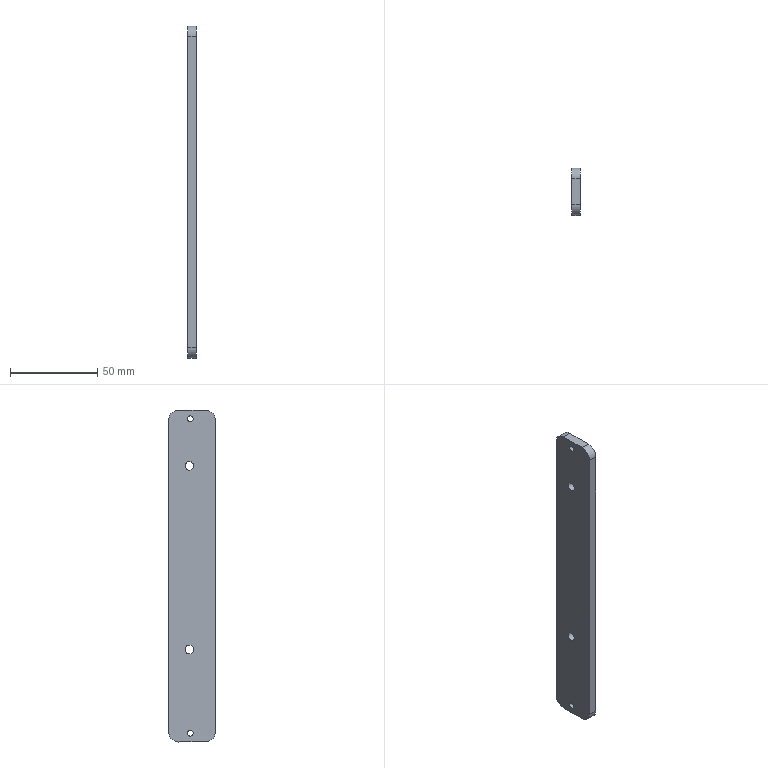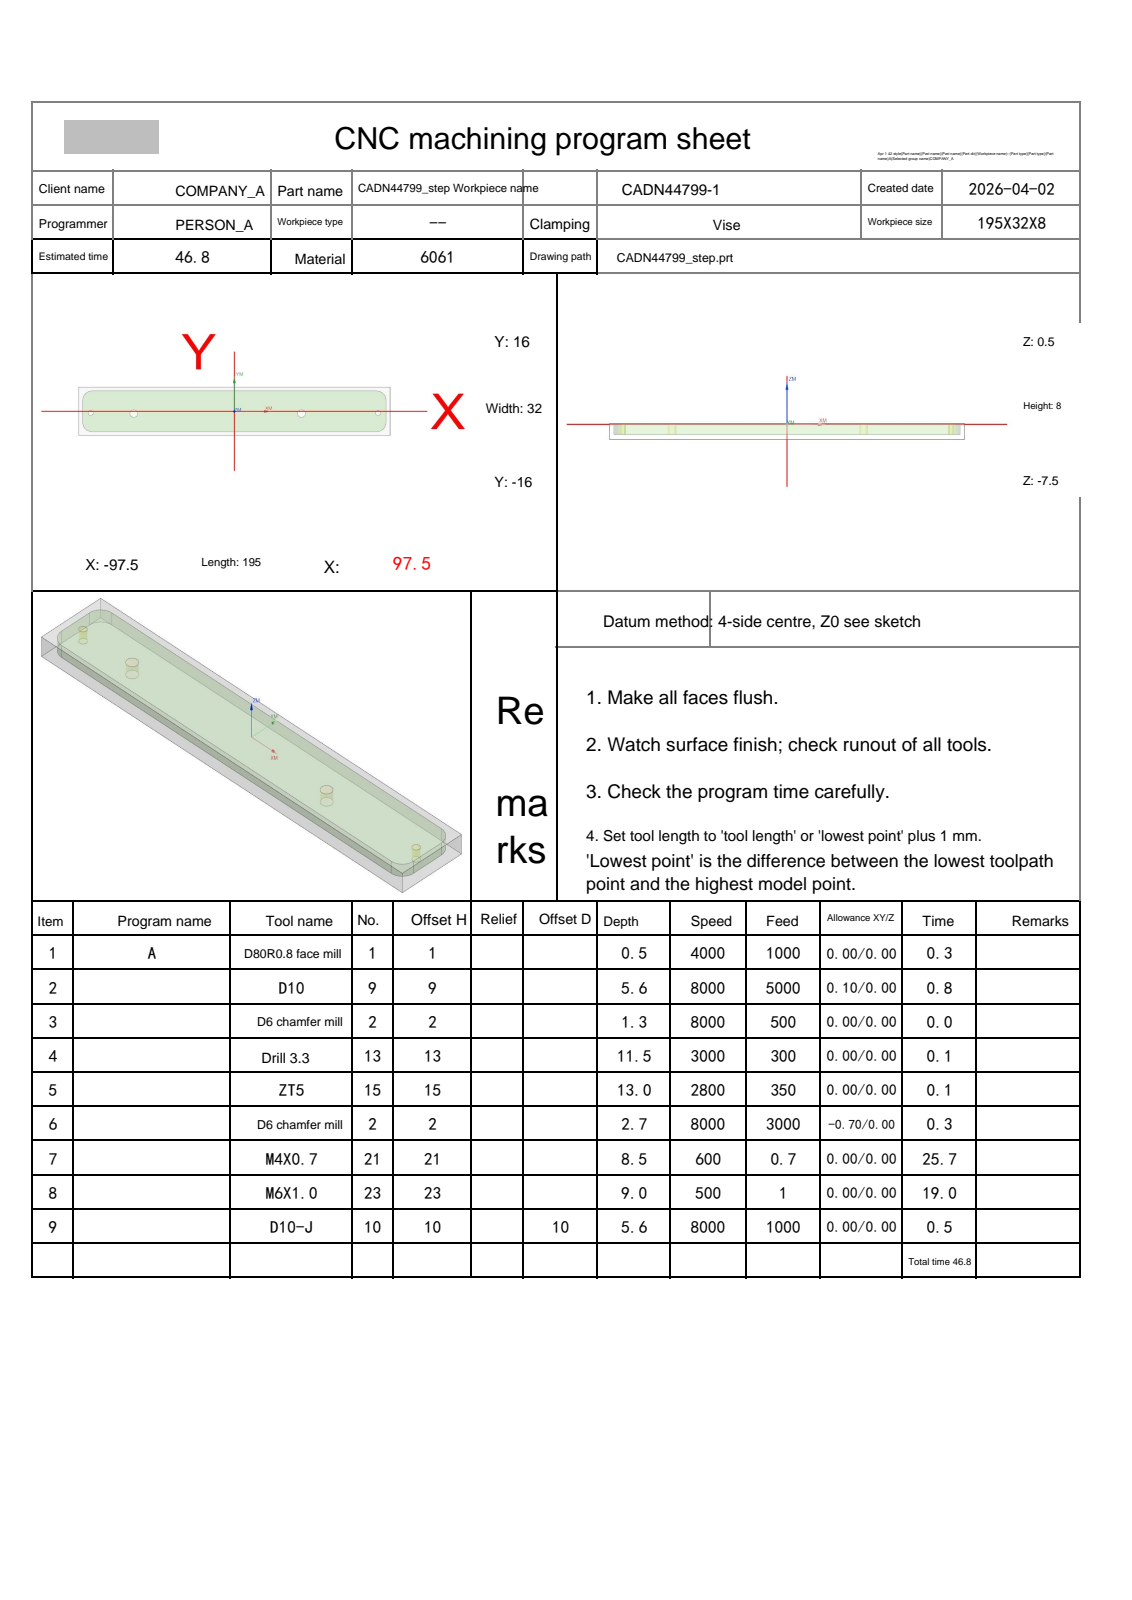NC program | NX | posted by the shop | part box 5 x 27 x 190 mm
Whole program:
%
O0001
(Machine time: 88.55 MIN)
(===Total Tool:8===)
(T1=D80R0.8 face mill D=80.  R=0.8  D-  H01 Z=-0.   )
(T9=D10     D=10.  R=0.   D-  H09 Z=-5.1  )
(T2=D6 chamfer mill   D=6.   R=0.   D-  H02 Z=-2.2  )
(T13=drill 3.3  D=3.3  DR_a=118 D-  H13 Z=-10.99)
(T15=ZT5    D=5.   DR_a=118 D-  H15 Z=-12.5 )
(T21=M4X0.7 D=3.3  DR_a=180 D-  H21 Z=-8.   )
(T23=M6X1.0 D=5.   DR_a=180 D-  H23 Z=-8.5  )
(T10=D10-J  D=10.  R=0.   D10 H10 Z=-5.1  )
G80 G90 G17 G49 G40
G91 G28 Z0
M01
N1 T01 M06
(D80R0.8 face mill  D=80. R=0.8 H=01 ce=0.00 di=0.00)
G00 G90 G54 X140. Y0.0 M03 S4000
G43 H01 Z20.
M08
Z2.
G01 Z0.0 F1000.
X135.
X-135.
X-140.
Z2.
G00 Z20.
G91 G28 Z0.0
M05
M09
G91 G28 Z0.0
M01
N2 T09 M06
(D10  D=10. R=0. H=09 ce=0.10 di=0.00)
G00 G90 G54 X0.0 Y-18.6 M03 S8000
G43 H09 Z20.
M08
Z.5
G01 X-89. Z.363 F5000.
G02 X-100.1 Y-7.5 Z.337 I0.0 J11.1
G01 Y7.5 Z.313
G02 X-89. Y18.6 Z.287 I11.1 J0.0
G01 X89. Z.013
G02 X100.1 Y7.5 Z-.013 I0.0 J-11.1
G01 Y-7.5 Z-.037
G02 X89. Y-18.6 Z-.063 I-11.1 J0.0
G01 X-89. Z-.337
G02 X-100.1 Y-7.5 Z-.363 I0.0 J11.1
G01 Y7.5 Z-.387
G02 X-89. Y18.6 Z-.413 I11.1 J0.0
G01 X89. Z-.687
G02 X100.1 Y7.5 Z-.713 I0.0 J-11.1
G01 Y-7.5 Z-.737
G02 X89. Y-18.6 Z-.763 I-11.1 J0.0
G01 X-89. Z-1.037
G02 X-100.1 Y-7.5 Z-1.063 I0.0 J11.1
G01 Y7.5 Z-1.087
G02 X-89. Y18.6 Z-1.113 I11.1 J0.0
G01 X89. Z-1.387
G02 X100.1 Y7.5 Z-1.413 I0.0 J-11.1
G01 Y-7.5 Z-1.437
G02 X89. Y-18.6 Z-1.463 I-11.1 J0.0
G01 X-89. Z-1.737
G02 X-100.1 Y-7.5 Z-1.763 I0.0 J11.1
G01 Y7.5 Z-1.787
G02 X-89. Y18.6 Z-1.813 I11.1 J0.0
G01 X89. Z-2.087
G02 X100.1 Y7.5 Z-2.113 I0.0 J-11.1
G01 Y-7.5 Z-2.137
G02 X89. Y-18.6 Z-2.163 I-11.1 J0.0
G01 X-89. Z-2.437
G02 X-100.1 Y-7.5 Z-2.463 I0.0 J11.1
G01 Y7.5 Z-2.487
G02 X-89. Y18.6 Z-2.513 I11.1 J0.0
G01 X89. Z-2.787
G02 X100.1 Y7.5 Z-2.813 I0.0 J-11.1
G01 Y-7.5 Z-2.837
G02 X89. Y-18.6 Z-2.863 I-11.1 J0.0
G01 X-89. Z-3.137
G02 X-100.1 Y-7.5 Z-3.163 I0.0 J11.1
G01 Y7.5 Z-3.187
G02 X-89. Y18.6 Z-3.213 I11.1 J0.0
G01 X89. Z-3.487
G02 X100.1 Y7.5 Z-3.513 I0.0 J-11.1
G01 Y-7.5 Z-3.537
G02 X89. Y-18.6 Z-3.563 I-11.1 J0.0
G01 X-89. Z-3.837
G02 X-100.1 Y-7.5 Z-3.863 I0.0 J11.1
G01 Y7.5 Z-3.887
G02 X-89. Y18.6 Z-3.913 I11.1 J0.0
G01 X89. Z-4.187
G02 X100.1 Y7.5 Z-4.213 I0.0 J-11.1
G01 Y-7.5 Z-4.237
G02 X89. Y-18.6 Z-4.263 I-11.1 J0.0
G01 X-89. Z-4.537
G02 X-100.1 Y-7.5 Z-4.563 I0.0 J11.1
G01 Y7.5 Z-4.587
G02 X-89. Y18.6 Z-4.613 I11.1 J0.0
G01 X89. Z-4.887
G02 X100.1 Y7.5 Z-4.913 I0.0 J-11.1
G01 Y-7.5 Z-4.937
G02 X89. Y-18.6 Z-4.963 I-11.1 J0.0
G01 X0.0 Z-5.1
X-89.
G02 X-100.1 Y-7.5 I0.0 J11.1
G01 Y7.5
G02 X-89. Y18.6 I11.1 J0.0
G01 X89.
G02 X100.1 Y7.5 I0.0 J-11.1
G01 Y-7.5
G02 X89. Y-18.6 I-11.1 J0.0
G01 X0.0
X-.5
Z-4.1
G00 Z20.
G91 G28 Z0.0
M05
M09
G91 G28 Z0.0
M01
N3 T02 M06
(D6 chamfer mill  D=6. R=0. H=02 ce=0.00 di=0.00)
G00 G90 G54 X-90.005 Y-1. M03 S8000
G43 H02 Z20.
M08
G98 G81 X-90.005 Y-1. Z-.8 R1. F500.
X-63.001 Y-1.454
X42.043
X89.995 Y-1.
G80
G00 Z20.
G91 G28 Z0.0
M05
M09
G91 G28 Z0.0
M01
N4 T13 M06
(drill 3.3 D=3.3 DR_a=118 H=13)
G00 G90 G54 X-90.005 Y-1. M03 S3000
G43 H13 Z20.
M08
G98 G83 X-90.005 Y-1. Z-10.991 R1. F300. Q2.
X89.995
G80
G00 Z20.
G91 G28 Z0.0
M05
M09
G91 G28 Z0.0
M01
N5 T15 M06
(ZT5 D=5. DR_a=118 H=15)
G00 G90 G54 X-63.001 Y-1.454 M03 S2800
G43 H15 Z20.
M08
G98 G83 X-63.001 Y-1.454 Z-12.502 R1. F350. Q3.
X42.043
G80
G00 Z20.
G91 G28 Z0.0
M05
M09
G91 G28 Z0.0
M01
N6 T02 M06
(D6 chamfer mill  D=6. R=0. H=02 ce=0.00 di=0.00)
G00 G90 G54 X.25 Y-15.628 M03 S8000
G43 H02 Z20.
M08
Z2.099
G01 Z-1.499 F3000.
G03 X.33 Y-15.328 I-.52 J.3
X.03 Y-14.808 I-.6 J0.0
G01 X0.0 Y-14.8
X-89.
G02 X-96.3 Y-7.5 I0.0 J7.3
G01 Y7.5
G02 X-89. Y14.8 I7.3 J0.0
G01 X89.
G02 X96.3 Y7.5 I0.0 J-7.3
G01 Y-7.5
G02 X89. Y-14.8 I-7.3 J0.0
G01 X0.0
X-.03 Y-14.808
G03 X-.33 Y-15.328 I.3 J-.52
X-.25 Y-15.628 I.6 J0.0
G01 Z2.099
G00 Z20.
G00 G90 X-90.005 Y-1. M03 S8000
Z20.
G98 G81 X-90.005 Y-1. Z-2.2 R3. F500.
X89.995
G80
G00 Z20.
G00 G90 X-63.409 Y-.433 M03 S8000
Z20.
Z-.6
G01 Z-1.1 F500.
X-63.601 Y.046
G03 X-65.101 Y-1.454 I0.0 J-1.5
X-63.001 Y-3.554 I2.1 J0.0
X-60.901 Y-1.454 I0.0 J2.1
X-63.001 Y.646 I-2.1 J0.0
X-65.101 Y-1.454 I0.0 J-2.1
X-63.601 Y-2.954 I1.5 J0.0
G01 X-63.409 Y-2.475
Z-.6
G00 Z20.
X41.635 Y-.433
Z-.6
G01 Z-1.1
X41.443 Y.046
G03 X39.943 Y-1.454 I0.0 J-1.5
X42.043 Y-3.554 I2.1 J0.0
X44.143 Y-1.454 I0.0 J2.1
X42.043 Y.646 I-2.1 J0.0
X39.943 Y-1.454 I0.0 J-2.1
X41.443 Y-2.954 I1.5 J0.0
G01 X41.635 Y-2.475
Z-.6
G00 Z20.
G91 G28 Z0.0
M05
M09
G91 G28 Z0.0
M01
N7 T21 M06
(M4X0.7 D=3.3 DR_a=180 H=21)
G00 G90 G54 X-90.005 Y-1. M03 S600
G43 H21 Z20.
M08
G95
G98 G84 X-90.005 Y-1. Z-8. R1. F.7 Q4.
X89.995
G80
G94
G00 Z20.
G91 G28 Z0.0
M05
M09
G91 G28 Z0.0
M01
N8 T23 M06
(M6X1.0 D=5. DR_a=180 H=23)
G00 G90 G54 X-63.001 Y-1.454 M03 S500
G43 H23 Z20.
M08
G95
G98 G84 X-63.001 Y-1.454 Z-8.5 R1. F1. Q3.
X42.043
G80
G94
G00 Z20.
G91 G28 Z0.0
M05
M09
G91 G28 Z0.0
M01
N9 T10 M06
(D10-J  D=10. R=0. H=10 ce=0.00 di=0.00)
G00 G90 G54 X90.007 Y-19.658 M03 S8000
G43 H10 Z20.
M08
Z-4.6
G01 Z-5.1 F1000.
G41 D10
X89.999 Y-19.458
G03 X89. Y-18.5 I-.999 J-.042
G01 X-89.
G02 X-100. Y-7.5 I0.0 J11.
G01 Y7.5
G02 X-89. Y18.5 I11. J0.0
G01 X89.
G02 X100. Y7.5 I0.0 J-11.
G01 Y-7.5
G02 X89. Y-18.5 I-11. J0.0
G01 X88.5
G03 X87.5 Y-19.5 I0.0 J-1.
G01 G40 Y-19.7
Z-4.6
G00 Z20.
M05
M09
G91 G28 Z0.0
G91 G28 Y0.0
M30
%